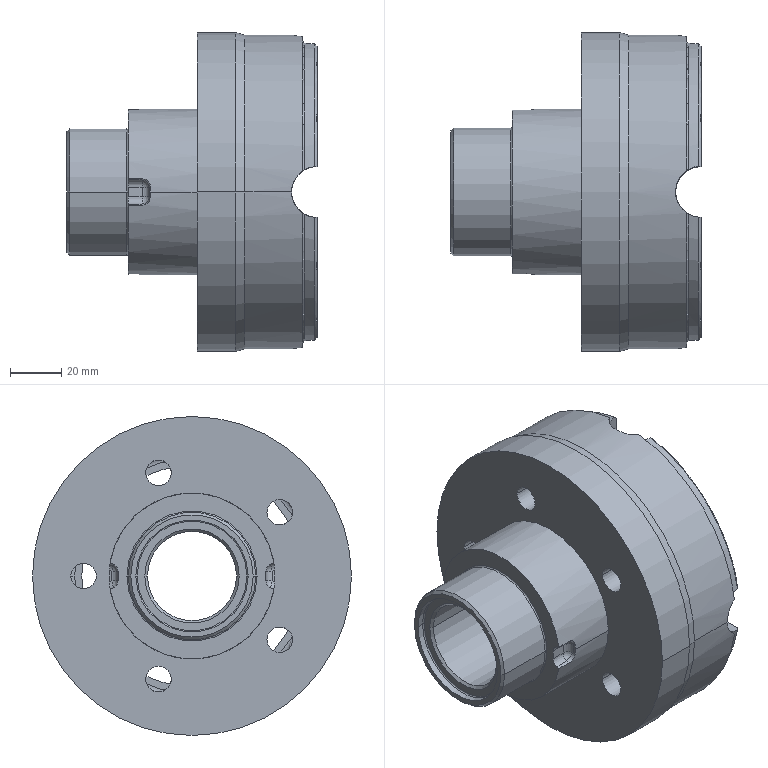Part | SolidWorks | features Fillet 5, Cut 4, Draft 3, ICE 3, CirPattern 2, Chamfer 1, HoleWzd 1, Revolution 1 | 1 solid | 173 faces | box 98 x 125 x 125 mm | volume 341274 mm3 | cylinder 64 | cone 48 | plane 37 | torus 18 | sphere 6 | commonest cylinder face diameters 6.8 x16 6 x10 10 x10 20 x4 50 x4 118 x4